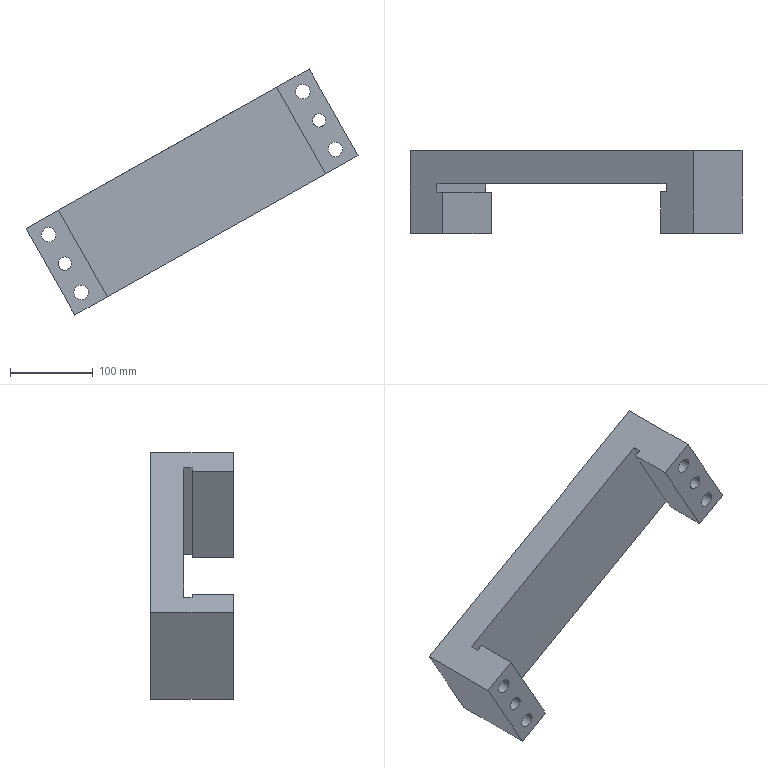Part | STEP file | solid 152 | 1 solid | 28 faces | box 400.456 x 100 x 296.842 mm | volume 2354176 mm3 | plane 15 | cylinder 10 | spline 3 | commonest cylinder face diameters 17.5 x4 26 x4 16 x2